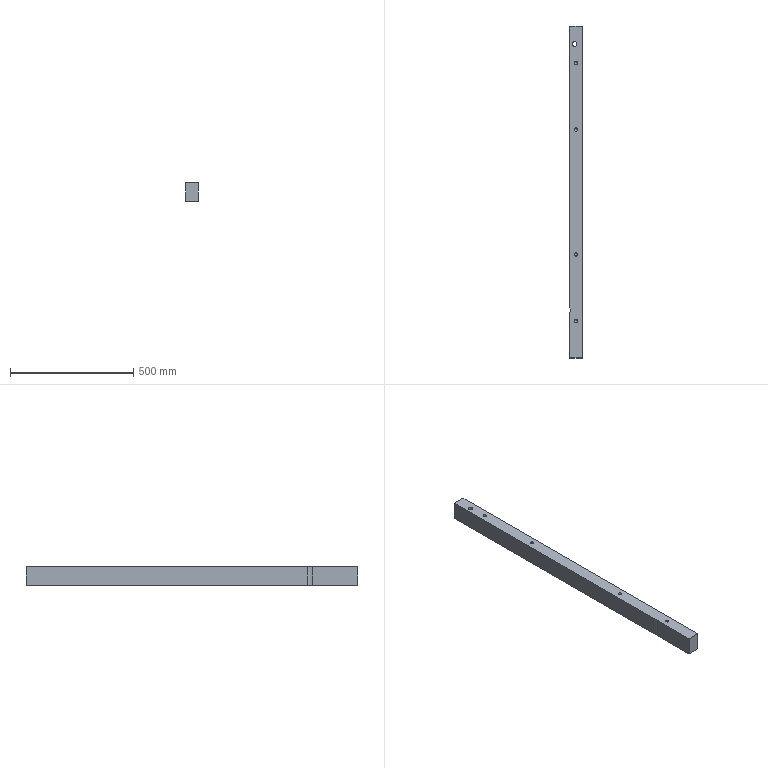Part | NX | features 3 2 | 1 solid | 25 faces | box 50 x 1345 x 75.5 mm | volume 5043227 mm3 | cylinder 10 | cone 8 | plane 7 | commonest cylinder face diameters 14.1 x8 18 x1 54 x1
STEP:
#1=CARTESIAN_POINT('',(1077.05,-522.5,256.5));
#2=VERTEX_POINT('',#1);
#3=CARTESIAN_POINT('',(1070.,-522.5,256.5));
#4=DIRECTION('',(0.,0.,-1.));
#5=DIRECTION('',(1.,0.,0.));
#6=AXIS2_PLACEMENT_3D('',#3,#4,#5);
#7=CIRCLE('',#6,7.05);
#8=EDGE_CURVE('',#2,#2,#7,.T.);
#9=ORIENTED_EDGE('',*,*,#8,.T.);
#10=EDGE_LOOP('',(#9));
#11=FACE_BOUND('',#10,.T.);
#12=CARTESIAN_POINT('',(1077.05,-252.5,256.5));
#13=VERTEX_POINT('',#12);
#14=CARTESIAN_POINT('',(1070.,-252.5,256.5));
#15=DIRECTION('',(0.,0.,-1.));
#16=DIRECTION('',(1.,0.,0.));
#17=AXIS2_PLACEMENT_3D('',#14,#15,#16);
#18=CIRCLE('',#17,7.05);
#19=EDGE_CURVE('',#13,#13,#18,.T.);
#20=ORIENTED_EDGE('',*,*,#19,.T.);
#21=EDGE_LOOP('',(#20));
#22=FACE_BOUND('',#21,.T.);
#23=CARTESIAN_POINT('',(1045.,-490.198,256.5));
#24=VERTEX_POINT('',#23);
#25=CARTESIAN_POINT('',(1045.,-469.802,256.5));
#26=VERTEX_POINT('',#25);
#27=CARTESIAN_POINT('',(1020.,-480.,256.5));
#28=DIRECTION('',(0.,0.,1.));
#29=DIRECTION('',(1.,0.,0.));
#30=AXIS2_PLACEMENT_3D('',#27,#28,#29);
#31=CIRCLE('',#30,27.);
#32=EDGE_CURVE('',#24,#26,#31,.T.);
#33=ORIENTED_EDGE('',*,*,#32,.F.);
#34=CARTESIAN_POINT('',(1045.,-672.5,256.5));
#35=VERTEX_POINT('',#34);
#36=CARTESIAN_POINT('',(1045.,193.,256.5));
#37=DIRECTION('',(0.,1.,0.));
#38=VECTOR('',#37,1000.);
#39=LINE('',#36,#38);
#40=EDGE_CURVE('',#35,#24,#39,.T.);
#41=ORIENTED_EDGE('',*,*,#40,.F.);
#42=CARTESIAN_POINT('',(1095.,-672.5,256.5));
#43=VERTEX_POINT('',#42);
#44=CARTESIAN_POINT('',(222.5,-672.5,256.5));
#45=DIRECTION('',(-1.,0.,0.));
#46=VECTOR('',#45,1000.);
#47=LINE('',#44,#46);
#48=EDGE_CURVE('',#43,#35,#47,.T.);
#49=ORIENTED_EDGE('',*,*,#48,.F.);
#50=CARTESIAN_POINT('',(1095.,672.5,256.5));
#51=VERTEX_POINT('',#50);
#52=CARTESIAN_POINT('',(1095.,193.,256.5));
#53=DIRECTION('',(0.,-1.,0.));
#54=VECTOR('',#53,1000.);
#55=LINE('',#52,#54);
#56=EDGE_CURVE('',#51,#43,#55,.T.);
#57=ORIENTED_EDGE('',*,*,#56,.F.);
#58=CARTESIAN_POINT('',(1045.,672.5,256.5));
#59=VERTEX_POINT('',#58);
#60=CARTESIAN_POINT('',(3085.,672.5,256.5));
#61=DIRECTION('',(-1.,0.,0.));
#62=VECTOR('',#61,1000.);
#63=LINE('',#60,#62);
#64=EDGE_CURVE('',#51,#59,#63,.T.);
#65=ORIENTED_EDGE('',*,*,#64,.T.);
#66=CARTESIAN_POINT('',(1045.,193.,256.5));
#67=DIRECTION('',(0.,1.,0.));
#68=VECTOR('',#67,1000.);
#69=LINE('',#66,#68);
#70=EDGE_CURVE('',#26,#59,#69,.T.);
#71=ORIENTED_EDGE('',*,*,#70,.F.);
#72=EDGE_LOOP('',(#33,#41,#49,#57,#65,#71));
#73=FACE_BOUND('',#72,.T.);
#74=CARTESIAN_POINT('',(1074.,599.5,256.5));
#75=VERTEX_POINT('',#74);
#76=CARTESIAN_POINT('',(1065.,599.5,256.5));
#77=DIRECTION('',(0.,0.,1.));
#78=DIRECTION('',(1.,0.,0.));
#79=AXIS2_PLACEMENT_3D('',#76,#77,#78);
#80=CIRCLE('',#79,9.);
#81=EDGE_CURVE('',#75,#75,#80,.T.);
#82=ORIENTED_EDGE('',*,*,#81,.F.);
#83=EDGE_LOOP('',(#82));
#84=FACE_BOUND('',#83,.T.);
#85=CARTESIAN_POINT('',(1077.05,252.5,256.5));
#86=VERTEX_POINT('',#85);
#87=CARTESIAN_POINT('',(1070.,252.5,256.5));
#88=DIRECTION('',(0.,0.,-1.));
#89=DIRECTION('',(1.,0.,0.));
#90=AXIS2_PLACEMENT_3D('',#87,#88,#89);
#91=CIRCLE('',#90,7.05);
#92=EDGE_CURVE('',#86,#86,#91,.T.);
#93=ORIENTED_EDGE('',*,*,#92,.T.);
#94=EDGE_LOOP('',(#93));
#95=FACE_BOUND('',#94,.T.);
#96=CARTESIAN_POINT('',(1077.05,522.5,256.5));
#97=VERTEX_POINT('',#96);
#98=CARTESIAN_POINT('',(1070.,522.5,256.5));
#99=DIRECTION('',(0.,0.,-1.));
#100=DIRECTION('',(1.,0.,0.));
#101=AXIS2_PLACEMENT_3D('',#98,#99,#100);
#102=CIRCLE('',#101,7.05);
#103=EDGE_CURVE('',#97,#97,#102,.T.);
#104=ORIENTED_EDGE('',*,*,#103,.T.);
#105=EDGE_LOOP('',(#104));
#106=FACE_BOUND('',#105,.T.);
#107=CARTESIAN_POINT('',(3085.,0.,256.5));
#108=DIRECTION('',(0.,0.,1.));
#109=DIRECTION('',(-1.,0.,0.));
#110=AXIS2_PLACEMENT_3D('',#107,#108,#109);
#111=PLANE('',#110);
#112=ADVANCED_FACE('',(#11,#22,#73,#84,#95,#106),#111,.T.);
#113=CARTESIAN_POINT('',(1077.05,252.5,181.));
#114=VERTEX_POINT('',#113);
#115=CARTESIAN_POINT('',(1070.,252.5,181.));
#116=DIRECTION('',(0.,0.,1.));
#117=DIRECTION('',(1.,0.,0.));
#118=AXIS2_PLACEMENT_3D('',#115,#116,#117);
#119=CIRCLE('',#118,7.05);
#120=EDGE_CURVE('',#114,#114,#119,.T.);
#121=ORIENTED_EDGE('',*,*,#120,.T.);
#122=EDGE_LOOP('',(#121));
#123=FACE_BOUND('',#122,.T.);
#124=CARTESIAN_POINT('',(1077.05,-252.5,181.));
#125=VERTEX_POINT('',#124);
#126=CARTESIAN_POINT('',(1070.,-252.5,181.));
#127=DIRECTION('',(0.,0.,1.));
#128=DIRECTION('',(1.,0.,0.));
#129=AXIS2_PLACEMENT_3D('',#126,#127,#128);
#130=CIRCLE('',#129,7.05);
#131=EDGE_CURVE('',#125,#125,#130,.T.);
#132=ORIENTED_EDGE('',*,*,#131,.T.);
#133=EDGE_LOOP('',(#132));
#134=FACE_BOUND('',#133,.T.);
#135=CARTESIAN_POINT('',(1045.,-490.198,181.));
#136=VERTEX_POINT('',#135);
#137=CARTESIAN_POINT('',(1045.,-469.802,181.));
#138=VERTEX_POINT('',#137);
#139=CARTESIAN_POINT('',(1020.,-480.,181.));
#140=DIRECTION('',(0.,0.,1.));
#141=DIRECTION('',(-1.,0.,0.));
#142=AXIS2_PLACEMENT_3D('',#139,#140,#141);
#143=CIRCLE('',#142,27.);
#144=EDGE_CURVE('',#136,#138,#143,.T.);
#145=ORIENTED_EDGE('',*,*,#144,.T.);
#146=CARTESIAN_POINT('',(1045.,672.5,181.));
#147=VERTEX_POINT('',#146);
#148=CARTESIAN_POINT('',(1045.,193.,181.));
#149=DIRECTION('',(0.,-1.,0.));
#150=VECTOR('',#149,1000.);
#151=LINE('',#148,#150);
#152=EDGE_CURVE('',#147,#138,#151,.T.);
#153=ORIENTED_EDGE('',*,*,#152,.F.);
#154=CARTESIAN_POINT('',(1095.,672.5,181.));
#155=VERTEX_POINT('',#154);
#156=CARTESIAN_POINT('',(2315.,672.5,181.));
#157=DIRECTION('',(1.,0.,0.));
#158=VECTOR('',#157,1000.);
#159=LINE('',#156,#158);
#160=EDGE_CURVE('',#147,#155,#159,.T.);
#161=ORIENTED_EDGE('',*,*,#160,.T.);
#162=CARTESIAN_POINT('',(1095.,-672.5,181.));
#163=VERTEX_POINT('',#162);
#164=CARTESIAN_POINT('',(1095.,193.,181.));
#165=DIRECTION('',(0.,1.,0.));
#166=VECTOR('',#165,1000.);
#167=LINE('',#164,#166);
#168=EDGE_CURVE('',#163,#155,#167,.T.);
#169=ORIENTED_EDGE('',*,*,#168,.F.);
#170=CARTESIAN_POINT('',(1045.,-672.5,181.));
#171=VERTEX_POINT('',#170);
#172=CARTESIAN_POINT('',(2315.,-672.5,181.));
#173=DIRECTION('',(-1.,0.,0.));
#174=VECTOR('',#173,1000.);
#175=LINE('',#172,#174);
#176=EDGE_CURVE('',#163,#171,#175,.T.);
#177=ORIENTED_EDGE('',*,*,#176,.T.);
#178=CARTESIAN_POINT('',(1045.,193.,181.));
#179=DIRECTION('',(0.,-1.,0.));
#180=VECTOR('',#179,1000.);
#181=LINE('',#178,#180);
#182=EDGE_CURVE('',#136,#171,#181,.T.);
#183=ORIENTED_EDGE('',*,*,#182,.F.);
#184=EDGE_LOOP('',(#145,#153,#161,#169,#177,#183));
#185=FACE_BOUND('',#184,.T.);
#186=CARTESIAN_POINT('',(1056.,599.5,181.));
#187=VERTEX_POINT('',#186);
#188=CARTESIAN_POINT('',(1065.,599.5,181.));
#189=DIRECTION('',(0.,0.,-1.));
#190=DIRECTION('',(-1.,0.,0.));
#191=AXIS2_PLACEMENT_3D('',#188,#189,#190);
#192=CIRCLE('',#191,9.);
#193=EDGE_CURVE('',#187,#187,#192,.T.);
#194=ORIENTED_EDGE('',*,*,#193,.F.);
#195=EDGE_LOOP('',(#194));
#196=FACE_BOUND('',#195,.T.);
#197=CARTESIAN_POINT('',(1077.05,-522.5,181.));
#198=VERTEX_POINT('',#197);
#199=CARTESIAN_POINT('',(1070.,-522.5,181.));
#200=DIRECTION('',(0.,0.,1.));
#201=DIRECTION('',(1.,0.,0.));
#202=AXIS2_PLACEMENT_3D('',#199,#200,#201);
#203=CIRCLE('',#202,7.05);
#204=EDGE_CURVE('',#198,#198,#203,.T.);
#205=ORIENTED_EDGE('',*,*,#204,.T.);
#206=EDGE_LOOP('',(#205));
#207=FACE_BOUND('',#206,.T.);
#208=CARTESIAN_POINT('',(1077.05,522.5,181.));
#209=VERTEX_POINT('',#208);
#210=CARTESIAN_POINT('',(1070.,522.5,181.));
#211=DIRECTION('',(0.,0.,1.));
#212=DIRECTION('',(1.,0.,0.));
#213=AXIS2_PLACEMENT_3D('',#210,#211,#212);
#214=CIRCLE('',#213,7.05);
#215=EDGE_CURVE('',#209,#209,#214,.T.);
#216=ORIENTED_EDGE('',*,*,#215,.T.);
#217=EDGE_LOOP('',(#216));
#218=FACE_BOUND('',#217,.T.);
#219=CARTESIAN_POINT('',(2315.,193.,181.));
#220=DIRECTION('',(0.,0.,-1.));
#221=DIRECTION('',(-1.,0.,0.));
#222=AXIS2_PLACEMENT_3D('',#219,#220,#221);
#223=PLANE('',#222);
#224=ADVANCED_FACE('',(#123,#134,#185,#196,#207,#218),#223,.T.);
#225=CARTESIAN_POINT('',(1045.,-490.198,-181.));
#226=DIRECTION('',(0.,0.,-1.));
#227=VECTOR('',#226,1000.);
#228=LINE('',#225,#227);
#229=EDGE_CURVE('',#24,#136,#228,.T.);
#230=ORIENTED_EDGE('',*,*,#229,.T.);
#231=ORIENTED_EDGE('',*,*,#182,.T.);
#232=CARTESIAN_POINT('',(1045.,-672.5,-1.5));
#233=DIRECTION('',(0.,0.,1.));
#234=VECTOR('',#233,1000.);
#235=LINE('',#232,#234);
#236=EDGE_CURVE('',#171,#35,#235,.T.);
#237=ORIENTED_EDGE('',*,*,#236,.T.);
#238=ORIENTED_EDGE('',*,*,#40,.T.);
#239=EDGE_LOOP('',(#230,#231,#237,#238));
#240=FACE_BOUND('',#239,.T.);
#241=CARTESIAN_POINT('',(1045.,193.,-1.5));
#242=DIRECTION('',(-1.,0.,0.));
#243=DIRECTION('',(0.,0.,-1.));
#244=AXIS2_PLACEMENT_3D('',#241,#242,#243);
#245=PLANE('',#244);
#246=ADVANCED_FACE('',(#240),#245,.T.);
#247=ORIENTED_EDGE('',*,*,#64,.F.);
#248=CARTESIAN_POINT('',(1095.,672.5,-1.5));
#249=DIRECTION('',(0.,0.,1.));
#250=VECTOR('',#249,1000.);
#251=LINE('',#248,#250);
#252=EDGE_CURVE('',#155,#51,#251,.T.);
#253=ORIENTED_EDGE('',*,*,#252,.F.);
#254=ORIENTED_EDGE('',*,*,#160,.F.);
#255=CARTESIAN_POINT('',(1045.,672.5,-1.5));
#256=DIRECTION('',(0.,0.,-1.));
#257=VECTOR('',#256,1000.);
#258=LINE('',#255,#257);
#259=EDGE_CURVE('',#59,#147,#258,.T.);
#260=ORIENTED_EDGE('',*,*,#259,.F.);
#261=EDGE_LOOP('',(#247,#253,#254,#260));
#262=FACE_BOUND('',#261,.T.);
#263=CARTESIAN_POINT('',(282.5,672.5,101.));
#264=DIRECTION('',(0.,-1.,0.));
#265=DIRECTION('',(-1.,0.,0.));
#266=AXIS2_PLACEMENT_3D('',#263,#264,#265);
#267=PLANE('',#266);
#268=ADVANCED_FACE('',(#262),#267,.F.);
#269=CARTESIAN_POINT('',(1045.,-469.802,-181.));
#270=DIRECTION('',(0.,0.,1.));
#271=VECTOR('',#270,1000.);
#272=LINE('',#269,#271);
#273=EDGE_CURVE('',#138,#26,#272,.T.);
#274=ORIENTED_EDGE('',*,*,#273,.T.);
#275=ORIENTED_EDGE('',*,*,#70,.T.);
#276=ORIENTED_EDGE('',*,*,#259,.T.);
#277=ORIENTED_EDGE('',*,*,#152,.T.);
#278=EDGE_LOOP('',(#274,#275,#276,#277));
#279=FACE_BOUND('',#278,.T.);
#280=CARTESIAN_POINT('',(1045.,193.,-1.5));
#281=DIRECTION('',(-1.,0.,0.));
#282=DIRECTION('',(0.,0.,-1.));
#283=AXIS2_PLACEMENT_3D('',#280,#281,#282);
#284=PLANE('',#283);
#285=ADVANCED_FACE('',(#279),#284,.T.);
#286=ORIENTED_EDGE('',*,*,#168,.T.);
#287=ORIENTED_EDGE('',*,*,#252,.T.);
#288=ORIENTED_EDGE('',*,*,#56,.T.);
#289=CARTESIAN_POINT('',(1095.,-672.5,-1.5));
#290=DIRECTION('',(0.,0.,-1.));
#291=VECTOR('',#290,1000.);
#292=LINE('',#289,#291);
#293=EDGE_CURVE('',#43,#163,#292,.T.);
#294=ORIENTED_EDGE('',*,*,#293,.T.);
#295=EDGE_LOOP('',(#286,#287,#288,#294));
#296=FACE_BOUND('',#295,.T.);
#297=CARTESIAN_POINT('',(1095.,193.,-1.5));
#298=DIRECTION('',(1.,0.,0.));
#299=DIRECTION('',(0.,0.,1.));
#300=AXIS2_PLACEMENT_3D('',#297,#298,#299);
#301=PLANE('',#300);
#302=ADVANCED_FACE('',(#296),#301,.T.);
#303=ORIENTED_EDGE('',*,*,#293,.F.);
#304=ORIENTED_EDGE('',*,*,#48,.T.);
#305=ORIENTED_EDGE('',*,*,#236,.F.);
#306=ORIENTED_EDGE('',*,*,#176,.F.);
#307=EDGE_LOOP('',(#303,#304,#305,#306));
#308=FACE_BOUND('',#307,.T.);
#309=CARTESIAN_POINT('',(222.5,-672.5,-103.));
#310=DIRECTION('',(0.,1.,0.));
#311=DIRECTION('',(1.,0.,0.));
#312=AXIS2_PLACEMENT_3D('',#309,#310,#311);
#313=PLANE('',#312);
#314=ADVANCED_FACE('',(#308),#313,.F.);
#315=ORIENTED_EDGE('',*,*,#81,.T.);
#316=EDGE_LOOP('',(#315));
#317=FACE_BOUND('',#316,.T.);
#318=ORIENTED_EDGE('',*,*,#193,.T.);
#319=EDGE_LOOP('',(#318));
#320=FACE_BOUND('',#319,.T.);
#321=CARTESIAN_POINT('',(1065.,599.5,-306.5));
#322=DIRECTION('',(0.,0.,1.));
#323=DIRECTION('',(-1.,0.,0.));
#324=AXIS2_PLACEMENT_3D('',#321,#322,#323);
#325=CYLINDRICAL_SURFACE('',#324,9.);
#326=ADVANCED_FACE('',(#317,#320),#325,.F.);
#327=ORIENTED_EDGE('',*,*,#229,.F.);
#328=ORIENTED_EDGE('',*,*,#32,.T.);
#329=ORIENTED_EDGE('',*,*,#273,.F.);
#330=ORIENTED_EDGE('',*,*,#144,.F.);
#331=EDGE_LOOP('',(#327,#328,#329,#330));
#332=FACE_BOUND('',#331,.T.);
#333=CARTESIAN_POINT('',(1020.,-480.,-181.));
#334=DIRECTION('',(0.,0.,1.));
#335=DIRECTION('',(-1.,0.,0.));
#336=AXIS2_PLACEMENT_3D('',#333,#334,#335);
#337=CYLINDRICAL_SURFACE('',#336,27.);
#338=ADVANCED_FACE('',(#332),#337,.F.);
#339=CARTESIAN_POINT('',(1077.05,-252.5,188.95));
#340=VERTEX_POINT('',#339);
#341=CARTESIAN_POINT('',(1070.,-252.5,188.95));
#342=DIRECTION('',(0.,0.,1.));
#343=DIRECTION('',(1.,0.,0.));
#344=AXIS2_PLACEMENT_3D('',#341,#342,#343);
#345=CIRCLE('',#344,7.05);
#346=EDGE_CURVE('',#340,#340,#345,.T.);
#347=ORIENTED_EDGE('',*,*,#346,.T.);
#348=EDGE_LOOP('',(#347));
#349=FACE_BOUND('',#348,.T.);
#350=ORIENTED_EDGE('',*,*,#131,.F.);
#351=EDGE_LOOP('',(#350));
#352=FACE_BOUND('',#351,.T.);
#353=CARTESIAN_POINT('',(1070.,-252.5,181.));
#354=DIRECTION('',(0.,0.,1.));
#355=DIRECTION('',(-1.,0.,0.));
#356=AXIS2_PLACEMENT_3D('',#353,#354,#355);
#357=CYLINDRICAL_SURFACE('',#356,7.05);
#358=ADVANCED_FACE('',(#349,#352),#357,.F.);
#359=CARTESIAN_POINT('',(1070.,-252.5,196.));
#360=VERTEX_POINT('',#359);
#361=VERTEX_LOOP('',#360);
#362=FACE_BOUND('',#361,.T.);
#363=ORIENTED_EDGE('',*,*,#346,.F.);
#364=EDGE_LOOP('',(#363));
#365=FACE_BOUND('',#364,.T.);
#366=CARTESIAN_POINT('',(1070.,-252.5,188.95));
#367=DIRECTION('',(0.,0.,-1.));
#368=DIRECTION('',(1.,0.,0.));
#369=AXIS2_PLACEMENT_3D('',#366,#367,#368);
#370=CONICAL_SURFACE('',#369,7.05,0.7854);
#371=ADVANCED_FACE('',(#362,#365),#370,.F.);
#372=CARTESIAN_POINT('',(1077.05,-522.5,188.95));
#373=VERTEX_POINT('',#372);
#374=CARTESIAN_POINT('',(1070.,-522.5,188.95));
#375=DIRECTION('',(0.,0.,1.));
#376=DIRECTION('',(1.,0.,0.));
#377=AXIS2_PLACEMENT_3D('',#374,#375,#376);
#378=CIRCLE('',#377,7.05);
#379=EDGE_CURVE('',#373,#373,#378,.T.);
#380=ORIENTED_EDGE('',*,*,#379,.T.);
#381=EDGE_LOOP('',(#380));
#382=FACE_BOUND('',#381,.T.);
#383=ORIENTED_EDGE('',*,*,#204,.F.);
#384=EDGE_LOOP('',(#383));
#385=FACE_BOUND('',#384,.T.);
#386=CARTESIAN_POINT('',(1070.,-522.5,181.));
#387=DIRECTION('',(0.,0.,1.));
#388=DIRECTION('',(-1.,0.,0.));
#389=AXIS2_PLACEMENT_3D('',#386,#387,#388);
#390=CYLINDRICAL_SURFACE('',#389,7.05);
#391=ADVANCED_FACE('',(#382,#385),#390,.F.);
#392=CARTESIAN_POINT('',(1070.,-522.5,196.));
#393=VERTEX_POINT('',#392);
#394=VERTEX_LOOP('',#393);
#395=FACE_BOUND('',#394,.T.);
#396=ORIENTED_EDGE('',*,*,#379,.F.);
#397=EDGE_LOOP('',(#396));
#398=FACE_BOUND('',#397,.T.);
#399=CARTESIAN_POINT('',(1070.,-522.5,188.95));
#400=DIRECTION('',(0.,0.,-1.));
#401=DIRECTION('',(1.,0.,0.));
#402=AXIS2_PLACEMENT_3D('',#399,#400,#401);
#403=CONICAL_SURFACE('',#402,7.05,0.7854);
#404=ADVANCED_FACE('',(#395,#398),#403,.F.);
#405=CARTESIAN_POINT('',(1077.05,252.5,188.95));
#406=VERTEX_POINT('',#405);
#407=CARTESIAN_POINT('',(1070.,252.5,188.95));
#408=DIRECTION('',(0.,0.,1.));
#409=DIRECTION('',(1.,0.,0.));
#410=AXIS2_PLACEMENT_3D('',#407,#408,#409);
#411=CIRCLE('',#410,7.05);
#412=EDGE_CURVE('',#406,#406,#411,.T.);
#413=ORIENTED_EDGE('',*,*,#412,.T.);
#414=EDGE_LOOP('',(#413));
#415=FACE_BOUND('',#414,.T.);
#416=ORIENTED_EDGE('',*,*,#120,.F.);
#417=EDGE_LOOP('',(#416));
#418=FACE_BOUND('',#417,.T.);
#419=CARTESIAN_POINT('',(1070.,252.5,181.));
#420=DIRECTION('',(0.,0.,1.));
#421=DIRECTION('',(-1.,0.,0.));
#422=AXIS2_PLACEMENT_3D('',#419,#420,#421);
#423=CYLINDRICAL_SURFACE('',#422,7.05);
#424=ADVANCED_FACE('',(#415,#418),#423,.F.);
#425=CARTESIAN_POINT('',(1070.,252.5,196.));
#426=VERTEX_POINT('',#425);
#427=VERTEX_LOOP('',#426);
#428=FACE_BOUND('',#427,.T.);
#429=ORIENTED_EDGE('',*,*,#412,.F.);
#430=EDGE_LOOP('',(#429));
#431=FACE_BOUND('',#430,.T.);
#432=CARTESIAN_POINT('',(1070.,252.5,188.95));
#433=DIRECTION('',(0.,0.,-1.));
#434=DIRECTION('',(1.,0.,0.));
#435=AXIS2_PLACEMENT_3D('',#432,#433,#434);
#436=CONICAL_SURFACE('',#435,7.05,0.7854);
#437=ADVANCED_FACE('',(#428,#431),#436,.F.);
#438=CARTESIAN_POINT('',(1077.05,522.5,188.95));
#439=VERTEX_POINT('',#438);
#440=CARTESIAN_POINT('',(1070.,522.5,188.95));
#441=DIRECTION('',(0.,0.,1.));
#442=DIRECTION('',(1.,0.,0.));
#443=AXIS2_PLACEMENT_3D('',#440,#441,#442);
#444=CIRCLE('',#443,7.05);
#445=EDGE_CURVE('',#439,#439,#444,.T.);
#446=ORIENTED_EDGE('',*,*,#445,.T.);
#447=EDGE_LOOP('',(#446));
#448=FACE_BOUND('',#447,.T.);
#449=ORIENTED_EDGE('',*,*,#215,.F.);
#450=EDGE_LOOP('',(#449));
#451=FACE_BOUND('',#450,.T.);
#452=CARTESIAN_POINT('',(1070.,522.5,181.));
#453=DIRECTION('',(0.,0.,1.));
#454=DIRECTION('',(-1.,0.,0.));
#455=AXIS2_PLACEMENT_3D('',#452,#453,#454);
#456=CYLINDRICAL_SURFACE('',#455,7.05);
#457=ADVANCED_FACE('',(#448,#451),#456,.F.);
#458=CARTESIAN_POINT('',(1070.,522.5,196.));
#459=VERTEX_POINT('',#458);
#460=VERTEX_LOOP('',#459);
#461=FACE_BOUND('',#460,.T.);
#462=ORIENTED_EDGE('',*,*,#445,.F.);
#463=EDGE_LOOP('',(#462));
#464=FACE_BOUND('',#463,.T.);
#465=CARTESIAN_POINT('',(1070.,522.5,188.95));
#466=DIRECTION('',(0.,0.,-1.));
#467=DIRECTION('',(1.,0.,0.));
#468=AXIS2_PLACEMENT_3D('',#465,#466,#467);
#469=CONICAL_SURFACE('',#468,7.05,0.7854);
#470=ADVANCED_FACE('',(#461,#464),#469,.F.);
#471=CARTESIAN_POINT('',(1062.95,-252.5,248.55));
#472=VERTEX_POINT('',#471);
#473=CARTESIAN_POINT('',(1070.,-252.5,248.55));
#474=DIRECTION('',(0.,0.,-1.));
#475=DIRECTION('',(-1.,0.,0.));
#476=AXIS2_PLACEMENT_3D('',#473,#474,#475);
#477=CIRCLE('',#476,7.05);
#478=EDGE_CURVE('',#472,#472,#477,.T.);
#479=ORIENTED_EDGE('',*,*,#478,.T.);
#480=EDGE_LOOP('',(#479));
#481=FACE_BOUND('',#480,.T.);
#482=ORIENTED_EDGE('',*,*,#19,.F.);
#483=EDGE_LOOP('',(#482));
#484=FACE_BOUND('',#483,.T.);
#485=CARTESIAN_POINT('',(1070.,-252.5,256.5));
#486=DIRECTION('',(0.,0.,-1.));
#487=DIRECTION('',(-1.,0.,0.));
#488=AXIS2_PLACEMENT_3D('',#485,#486,#487);
#489=CYLINDRICAL_SURFACE('',#488,7.05);
#490=ADVANCED_FACE('',(#481,#484),#489,.F.);
#491=CARTESIAN_POINT('',(1070.,-252.5,241.5));
#492=VERTEX_POINT('',#491);
#493=VERTEX_LOOP('',#492);
#494=FACE_BOUND('',#493,.T.);
#495=ORIENTED_EDGE('',*,*,#478,.F.);
#496=EDGE_LOOP('',(#495));
#497=FACE_BOUND('',#496,.T.);
#498=CARTESIAN_POINT('',(1070.,-252.5,248.55));
#499=DIRECTION('',(0.,0.,1.));
#500=DIRECTION('',(-1.,0.,0.));
#501=AXIS2_PLACEMENT_3D('',#498,#499,#500);
#502=CONICAL_SURFACE('',#501,7.05,0.7854);
#503=ADVANCED_FACE('',(#494,#497),#502,.F.);
#504=CARTESIAN_POINT('',(1062.95,252.5,248.55));
#505=VERTEX_POINT('',#504);
#506=CARTESIAN_POINT('',(1070.,252.5,248.55));
#507=DIRECTION('',(0.,0.,-1.));
#508=DIRECTION('',(-1.,0.,0.));
#509=AXIS2_PLACEMENT_3D('',#506,#507,#508);
#510=CIRCLE('',#509,7.05);
#511=EDGE_CURVE('',#505,#505,#510,.T.);
#512=ORIENTED_EDGE('',*,*,#511,.T.);
#513=EDGE_LOOP('',(#512));
#514=FACE_BOUND('',#513,.T.);
#515=ORIENTED_EDGE('',*,*,#92,.F.);
#516=EDGE_LOOP('',(#515));
#517=FACE_BOUND('',#516,.T.);
#518=CARTESIAN_POINT('',(1070.,252.5,256.5));
#519=DIRECTION('',(0.,0.,-1.));
#520=DIRECTION('',(-1.,0.,0.));
#521=AXIS2_PLACEMENT_3D('',#518,#519,#520);
#522=CYLINDRICAL_SURFACE('',#521,7.05);
#523=ADVANCED_FACE('',(#514,#517),#522,.F.);
#524=CARTESIAN_POINT('',(1070.,252.5,241.5));
#525=VERTEX_POINT('',#524);
#526=VERTEX_LOOP('',#525);
#527=FACE_BOUND('',#526,.T.);
#528=ORIENTED_EDGE('',*,*,#511,.F.);
#529=EDGE_LOOP('',(#528));
#530=FACE_BOUND('',#529,.T.);
#531=CARTESIAN_POINT('',(1070.,252.5,248.55));
#532=DIRECTION('',(0.,0.,1.));
#533=DIRECTION('',(-1.,0.,0.));
#534=AXIS2_PLACEMENT_3D('',#531,#532,#533);
#535=CONICAL_SURFACE('',#534,7.05,0.7854);
#536=ADVANCED_FACE('',(#527,#530),#535,.F.);
#537=CARTESIAN_POINT('',(1062.95,-522.5,248.55));
#538=VERTEX_POINT('',#537);
#539=CARTESIAN_POINT('',(1070.,-522.5,248.55));
#540=DIRECTION('',(0.,0.,-1.));
#541=DIRECTION('',(-1.,0.,0.));
#542=AXIS2_PLACEMENT_3D('',#539,#540,#541);
#543=CIRCLE('',#542,7.05);
#544=EDGE_CURVE('',#538,#538,#543,.T.);
#545=ORIENTED_EDGE('',*,*,#544,.T.);
#546=EDGE_LOOP('',(#545));
#547=FACE_BOUND('',#546,.T.);
#548=ORIENTED_EDGE('',*,*,#8,.F.);
#549=EDGE_LOOP('',(#548));
#550=FACE_BOUND('',#549,.T.);
#551=CARTESIAN_POINT('',(1070.,-522.5,256.5));
#552=DIRECTION('',(0.,0.,-1.));
#553=DIRECTION('',(-1.,0.,0.));
#554=AXIS2_PLACEMENT_3D('',#551,#552,#553);
#555=CYLINDRICAL_SURFACE('',#554,7.05);
#556=ADVANCED_FACE('',(#547,#550),#555,.F.);
#557=CARTESIAN_POINT('',(1070.,-522.5,241.5));
#558=VERTEX_POINT('',#557);
#559=VERTEX_LOOP('',#558);
#560=FACE_BOUND('',#559,.T.);
#561=ORIENTED_EDGE('',*,*,#544,.F.);
#562=EDGE_LOOP('',(#561));
#563=FACE_BOUND('',#562,.T.);
#564=CARTESIAN_POINT('',(1070.,-522.5,248.55));
#565=DIRECTION('',(0.,0.,1.));
#566=DIRECTION('',(-1.,0.,0.));
#567=AXIS2_PLACEMENT_3D('',#564,#565,#566);
#568=CONICAL_SURFACE('',#567,7.05,0.7854);
#569=ADVANCED_FACE('',(#560,#563),#568,.F.);
#570=CARTESIAN_POINT('',(1062.95,522.5,248.55));
#571=VERTEX_POINT('',#570);
#572=CARTESIAN_POINT('',(1070.,522.5,248.55));
#573=DIRECTION('',(0.,0.,-1.));
#574=DIRECTION('',(-1.,0.,0.));
#575=AXIS2_PLACEMENT_3D('',#572,#573,#574);
#576=CIRCLE('',#575,7.05);
#577=EDGE_CURVE('',#571,#571,#576,.T.);
#578=ORIENTED_EDGE('',*,*,#577,.T.);
#579=EDGE_LOOP('',(#578));
#580=FACE_BOUND('',#579,.T.);
#581=ORIENTED_EDGE('',*,*,#103,.F.);
#582=EDGE_LOOP('',(#581));
#583=FACE_BOUND('',#582,.T.);
#584=CARTESIAN_POINT('',(1070.,522.5,256.5));
#585=DIRECTION('',(0.,0.,-1.));
#586=DIRECTION('',(-1.,0.,0.));
#587=AXIS2_PLACEMENT_3D('',#584,#585,#586);
#588=CYLINDRICAL_SURFACE('',#587,7.05);
#589=ADVANCED_FACE('',(#580,#583),#588,.F.);
#590=CARTESIAN_POINT('',(1070.,522.5,241.5));
#591=VERTEX_POINT('',#590);
#592=VERTEX_LOOP('',#591);
#593=FACE_BOUND('',#592,.T.);
#594=ORIENTED_EDGE('',*,*,#577,.F.);
#595=EDGE_LOOP('',(#594));
#596=FACE_BOUND('',#595,.T.);
#597=CARTESIAN_POINT('',(1070.,522.5,248.55));
#598=DIRECTION('',(0.,0.,1.));
#599=DIRECTION('',(-1.,0.,0.));
#600=AXIS2_PLACEMENT_3D('',#597,#598,#599);
#601=CONICAL_SURFACE('',#600,7.05,0.7854);
#602=ADVANCED_FACE('',(#593,#596),#601,.F.);
#603=CLOSED_SHELL('',(#112,#224,#246,#268,#285,#302,#314,#326,#338,#358,#371,#391,#404,#424,#437,#457,#470,#490,#503,#523,#536,#556,#569,#589,#602));
#604=MANIFOLD_SOLID_BREP('',#603);
#605=(LENGTH_UNIT()NAMED_UNIT(*)SI_UNIT(.MILLI.,.METRE.));
#606=UNCERTAINTY_MEASURE_WITH_UNIT(LENGTH_MEASURE(0.00001),#605,'','');
#607=(NAMED_UNIT(*)PLANE_ANGLE_UNIT()SI_UNIT($,.RADIAN.));
#608=(NAMED_UNIT(*)SI_UNIT($,.STERADIAN.)SOLID_ANGLE_UNIT());
#609=(GEOMETRIC_REPRESENTATION_CONTEXT(3)GLOBAL_UNCERTAINTY_ASSIGNED_CONTEXT((#606))GLOBAL_UNIT_ASSIGNED_CONTEXT((#605,#607,#608))REPRESENTATION_CONTEXT('',''));
#610=ADVANCED_BREP_SHAPE_REPRESENTATION('',(#604),#609);